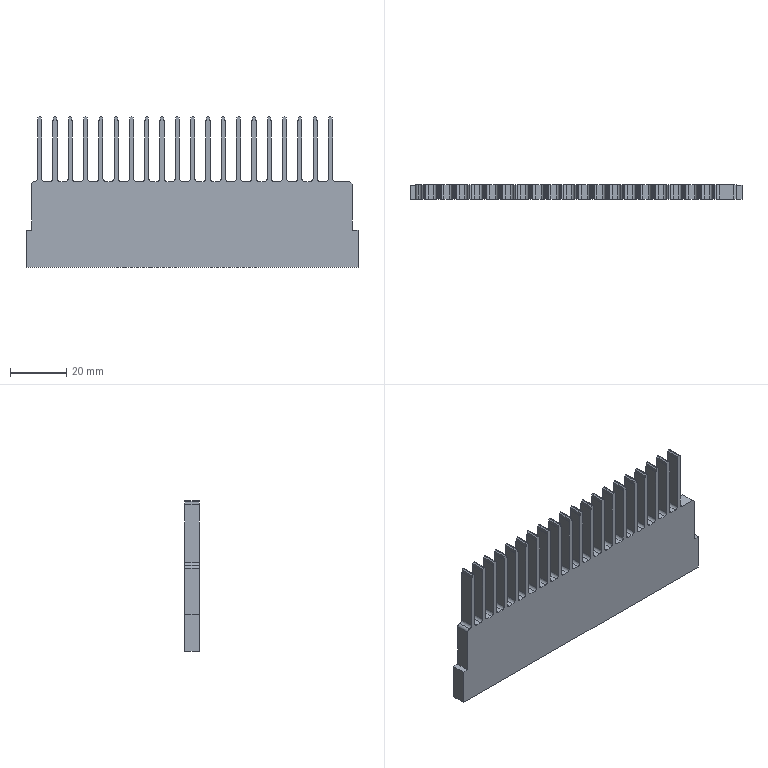Part | STEP file | 1 solid | 252 faces | box 118 x 5 x 53.54 mm | volume 21080 mm3 | plane 191 | cylinder 61 | commonest cylinder face diameters 2 x41 0.48 x20